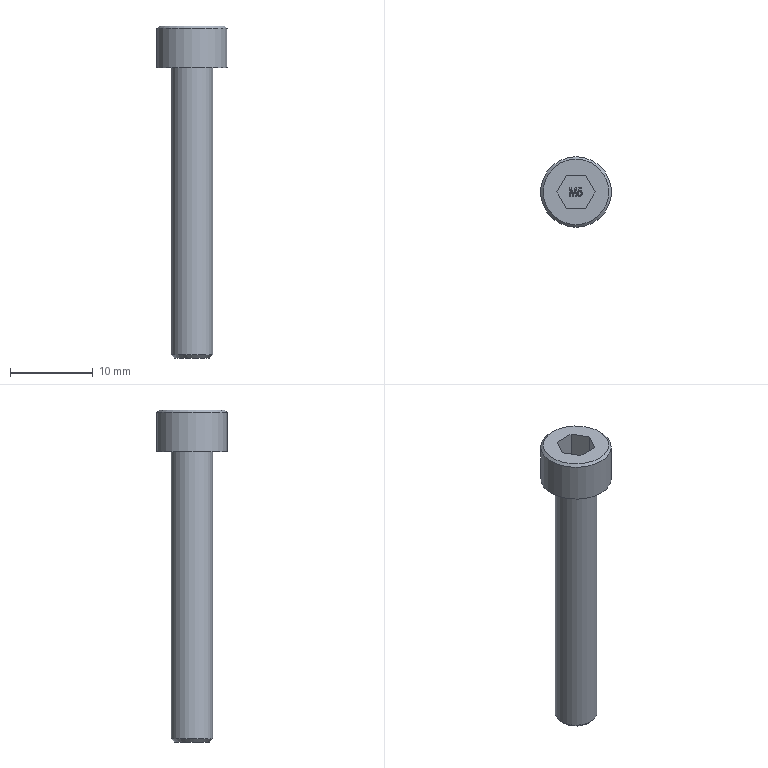Part | STEP file | EM10503500 | 1 solid | 39 faces | box 8.5 x 8.5 x 40 mm | volume 920.076 mm3 | plane 30 | other 5 | cylinder 2 | cone 2 | commonest cylinder face diameters 5 x1 8.5 x1